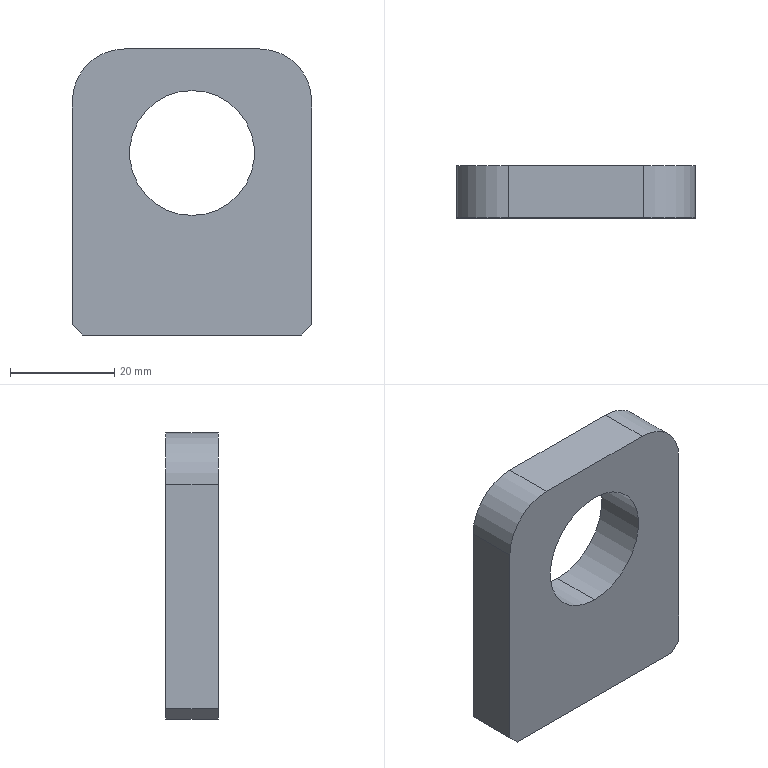Part | SolidWorks | features HoleWzd 2, Chamfer 1, Extrusion 1, Fillet 1 | 1 solid | 20 faces | box 46 x 10 x 55 mm | volume 20105 mm3 | cylinder 8 | plane 8 | cone 4 | commonest cylinder face diameters 3.3 x4 20 x2 24 x2
STEP:
#1=CARTESIAN_POINT('',(16.65,0.,-16.));
#2=VERTEX_POINT('',#1);
#3=CARTESIAN_POINT('',(13.35,0.,-16.));
#4=VERTEX_POINT('',#3);
#5=CARTESIAN_POINT('',(15.,0.,-16.));
#6=DIRECTION('',(0.,0.,-1.));
#7=DIRECTION('',(-1.,0.,0.));
#8=AXIS2_PLACEMENT_3D('',#5,#6,#7);
#9=CIRCLE('',#8,1.65);
#10=EDGE_CURVE('',#2,#4,#9,.T.);
#11=ORIENTED_EDGE('',*,*,#10,.F.);
#12=CARTESIAN_POINT('',(16.65,0.,-27.5));
#13=VERTEX_POINT('',#12);
#14=CARTESIAN_POINT('',(16.65,0.,-27.5));
#15=DIRECTION('',(0.,0.,-1.));
#16=VECTOR('',#15,1000.);
#17=LINE('',#14,#16);
#18=EDGE_CURVE('',#2,#13,#17,.T.);
#19=ORIENTED_EDGE('',*,*,#18,.T.);
#20=CARTESIAN_POINT('',(13.35,0.,-27.5));
#21=VERTEX_POINT('',#20);
#22=CARTESIAN_POINT('',(15.,0.,-27.5));
#23=DIRECTION('',(0.,0.,-1.));
#24=DIRECTION('',(-1.,0.,0.));
#25=AXIS2_PLACEMENT_3D('',#22,#23,#24);
#26=CIRCLE('',#25,1.65);
#27=EDGE_CURVE('',#13,#21,#26,.T.);
#28=ORIENTED_EDGE('',*,*,#27,.T.);
#29=CARTESIAN_POINT('',(13.35,0.,-27.5));
#30=DIRECTION('',(0.,0.,-1.));
#31=VECTOR('',#30,1000.);
#32=LINE('',#29,#31);
#33=EDGE_CURVE('',#4,#21,#32,.T.);
#34=ORIENTED_EDGE('',*,*,#33,.F.);
#35=EDGE_LOOP('',(#11,#19,#28,#34));
#36=FACE_OUTER_BOUND('',#35,.T.);
#37=CARTESIAN_POINT('',(15.,0.,-27.5));
#38=DIRECTION('',(0.,0.,-1.));
#39=DIRECTION('',(-1.,0.,0.));
#40=AXIS2_PLACEMENT_3D('',#37,#38,#39);
#41=CYLINDRICAL_SURFACE('',#40,1.65);
#42=ADVANCED_FACE('',(#36),#41,.F.);
#43=CARTESIAN_POINT('',(15.,0.,-15.009));
#44=VERTEX_POINT('',#43);
#45=CARTESIAN_POINT('',(13.35,0.,-16.));
#46=DIRECTION('',(-0.8572,0.,-0.515));
#47=VECTOR('',#46,1000.);
#48=LINE('',#45,#47);
#49=EDGE_CURVE('',#44,#4,#48,.T.);
#50=ORIENTED_EDGE('',*,*,#49,.F.);
#51=CARTESIAN_POINT('',(16.65,0.,-16.));
#52=DIRECTION('',(0.8572,0.,-0.515));
#53=VECTOR('',#52,1000.);
#54=LINE('',#51,#53);
#55=EDGE_CURVE('',#44,#2,#54,.T.);
#56=ORIENTED_EDGE('',*,*,#55,.T.);
#57=ORIENTED_EDGE('',*,*,#10,.T.);
#58=EDGE_LOOP('',(#50,#56,#57));
#59=FACE_OUTER_BOUND('',#58,.T.);
#60=CARTESIAN_POINT('',(15.,0.,-16.));
#61=DIRECTION('',(0.,0.,-1.));
#62=DIRECTION('',(-1.,0.,0.));
#63=AXIS2_PLACEMENT_3D('',#60,#61,#62);
#64=CONICAL_SURFACE('',#63,1.65,1.03);
#65=ADVANCED_FACE('',(#59),#64,.F.);
#66=CARTESIAN_POINT('',(-13.35,0.,-16.));
#67=VERTEX_POINT('',#66);
#68=CARTESIAN_POINT('',(-16.65,0.,-16.));
#69=VERTEX_POINT('',#68);
#70=CARTESIAN_POINT('',(-15.,0.,-16.));
#71=DIRECTION('',(0.,0.,-1.));
#72=DIRECTION('',(-1.,0.,0.));
#73=AXIS2_PLACEMENT_3D('',#70,#71,#72);
#74=CIRCLE('',#73,1.65);
#75=EDGE_CURVE('',#67,#69,#74,.T.);
#76=ORIENTED_EDGE('',*,*,#75,.F.);
#77=CARTESIAN_POINT('',(-13.35,0.,-27.5));
#78=VERTEX_POINT('',#77);
#79=CARTESIAN_POINT('',(-13.35,0.,-27.5));
#80=DIRECTION('',(0.,0.,-1.));
#81=VECTOR('',#80,1000.);
#82=LINE('',#79,#81);
#83=EDGE_CURVE('',#67,#78,#82,.T.);
#84=ORIENTED_EDGE('',*,*,#83,.T.);
#85=CARTESIAN_POINT('',(-16.65,0.,-27.5));
#86=VERTEX_POINT('',#85);
#87=CARTESIAN_POINT('',(-15.,0.,-27.5));
#88=DIRECTION('',(0.,0.,-1.));
#89=DIRECTION('',(-1.,0.,0.));
#90=AXIS2_PLACEMENT_3D('',#87,#88,#89);
#91=CIRCLE('',#90,1.65);
#92=EDGE_CURVE('',#78,#86,#91,.T.);
#93=ORIENTED_EDGE('',*,*,#92,.T.);
#94=CARTESIAN_POINT('',(-16.65,0.,-27.5));
#95=DIRECTION('',(0.,0.,-1.));
#96=VECTOR('',#95,1000.);
#97=LINE('',#94,#96);
#98=EDGE_CURVE('',#69,#86,#97,.T.);
#99=ORIENTED_EDGE('',*,*,#98,.F.);
#100=EDGE_LOOP('',(#76,#84,#93,#99));
#101=FACE_OUTER_BOUND('',#100,.T.);
#102=CARTESIAN_POINT('',(-15.,0.,-27.5));
#103=DIRECTION('',(0.,0.,-1.));
#104=DIRECTION('',(-1.,0.,0.));
#105=AXIS2_PLACEMENT_3D('',#102,#103,#104);
#106=CYLINDRICAL_SURFACE('',#105,1.65);
#107=ADVANCED_FACE('',(#101),#106,.F.);
#108=CARTESIAN_POINT('',(-15.,0.,-15.009));
#109=VERTEX_POINT('',#108);
#110=CARTESIAN_POINT('',(-16.65,0.,-16.));
#111=DIRECTION('',(-0.8572,0.,-0.515));
#112=VECTOR('',#111,1000.);
#113=LINE('',#110,#112);
#114=EDGE_CURVE('',#109,#69,#113,.T.);
#115=ORIENTED_EDGE('',*,*,#114,.F.);
#116=CARTESIAN_POINT('',(-13.35,0.,-16.));
#117=DIRECTION('',(0.8572,0.,-0.515));
#118=VECTOR('',#117,1000.);
#119=LINE('',#116,#118);
#120=EDGE_CURVE('',#109,#67,#119,.T.);
#121=ORIENTED_EDGE('',*,*,#120,.T.);
#122=ORIENTED_EDGE('',*,*,#75,.T.);
#123=EDGE_LOOP('',(#115,#121,#122));
#124=FACE_OUTER_BOUND('',#123,.T.);
#125=CARTESIAN_POINT('',(-15.,0.,-16.));
#126=DIRECTION('',(0.,0.,-1.));
#127=DIRECTION('',(-1.,0.,0.));
#128=AXIS2_PLACEMENT_3D('',#125,#126,#127);
#129=CONICAL_SURFACE('',#128,1.65,1.03);
#130=ADVANCED_FACE('',(#124),#129,.F.);
#131=CARTESIAN_POINT('',(0.,-5.,-4.5));
#132=VERTEX_POINT('',#131);
#133=CARTESIAN_POINT('',(0.,-5.,19.5));
#134=VERTEX_POINT('',#133);
#135=CARTESIAN_POINT('',(0.,-5.,7.5));
#136=DIRECTION('',(0.,1.,0.));
#137=DIRECTION('',(0.,0.,1.));
#138=AXIS2_PLACEMENT_3D('',#135,#136,#137);
#139=CIRCLE('',#138,12.);
#140=EDGE_CURVE('',#132,#134,#139,.T.);
#141=ORIENTED_EDGE('',*,*,#140,.F.);
#142=CARTESIAN_POINT('',(0.,5.,-4.5));
#143=VERTEX_POINT('',#142);
#144=CARTESIAN_POINT('',(0.,5.,-4.5));
#145=DIRECTION('',(0.,1.,0.));
#146=VECTOR('',#145,1000.);
#147=LINE('',#144,#146);
#148=EDGE_CURVE('',#132,#143,#147,.T.);
#149=ORIENTED_EDGE('',*,*,#148,.T.);
#150=CARTESIAN_POINT('',(0.,5.,19.5));
#151=VERTEX_POINT('',#150);
#152=CARTESIAN_POINT('',(0.,5.,7.5));
#153=DIRECTION('',(0.,1.,0.));
#154=DIRECTION('',(0.,0.,1.));
#155=AXIS2_PLACEMENT_3D('',#152,#153,#154);
#156=CIRCLE('',#155,12.);
#157=EDGE_CURVE('',#143,#151,#156,.T.);
#158=ORIENTED_EDGE('',*,*,#157,.T.);
#159=CARTESIAN_POINT('',(0.,5.,19.5));
#160=DIRECTION('',(0.,1.,0.));
#161=VECTOR('',#160,1000.);
#162=LINE('',#159,#161);
#163=EDGE_CURVE('',#134,#151,#162,.T.);
#164=ORIENTED_EDGE('',*,*,#163,.F.);
#165=EDGE_LOOP('',(#141,#149,#158,#164));
#166=FACE_OUTER_BOUND('',#165,.T.);
#167=CARTESIAN_POINT('',(0.,5.,7.5));
#168=DIRECTION('',(0.,1.,0.));
#169=DIRECTION('',(0.,0.,1.));
#170=AXIS2_PLACEMENT_3D('',#167,#168,#169);
#171=CYLINDRICAL_SURFACE('',#170,12.);
#172=ADVANCED_FACE('',(#166),#171,.F.);
#173=CARTESIAN_POINT('',(23.,-5.,17.5));
#174=VERTEX_POINT('',#173);
#175=CARTESIAN_POINT('',(23.,-5.,-25.5));
#176=VERTEX_POINT('',#175);
#177=CARTESIAN_POINT('',(23.,-5.,-27.5));
#178=DIRECTION('',(0.,0.,-1.));
#179=VECTOR('',#178,1000.);
#180=LINE('',#177,#179);
#181=EDGE_CURVE('',#174,#176,#180,.T.);
#182=ORIENTED_EDGE('',*,*,#181,.T.);
#183=CARTESIAN_POINT('',(23.,5.,-25.5));
#184=VERTEX_POINT('',#183);
#185=CARTESIAN_POINT('',(23.,5.,-25.5));
#186=DIRECTION('',(0.,1.,0.));
#187=VECTOR('',#186,1000.);
#188=LINE('',#185,#187);
#189=EDGE_CURVE('',#176,#184,#188,.T.);
#190=ORIENTED_EDGE('',*,*,#189,.T.);
#191=CARTESIAN_POINT('',(23.,5.,17.5));
#192=VERTEX_POINT('',#191);
#193=CARTESIAN_POINT('',(23.,5.,-27.5));
#194=DIRECTION('',(0.,0.,-1.));
#195=VECTOR('',#194,1000.);
#196=LINE('',#193,#195);
#197=EDGE_CURVE('',#192,#184,#196,.T.);
#198=ORIENTED_EDGE('',*,*,#197,.F.);
#199=CARTESIAN_POINT('',(23.,5.,17.5));
#200=DIRECTION('',(0.,-1.,0.));
#201=VECTOR('',#200,1000.);
#202=LINE('',#199,#201);
#203=EDGE_CURVE('',#192,#174,#202,.T.);
#204=ORIENTED_EDGE('',*,*,#203,.T.);
#205=EDGE_LOOP('',(#182,#190,#198,#204));
#206=FACE_OUTER_BOUND('',#205,.T.);
#207=CARTESIAN_POINT('',(23.,5.,-27.5));
#208=DIRECTION('',(-1.,0.,0.));
#209=DIRECTION('',(0.,0.,1.));
#210=AXIS2_PLACEMENT_3D('',#207,#208,#209);
#211=PLANE('',#210);
#212=ADVANCED_FACE('',(#206),#211,.F.);
#213=CARTESIAN_POINT('',(15.,0.,-27.5));
#214=DIRECTION('',(0.,0.,-1.));
#215=DIRECTION('',(-1.,0.,0.));
#216=AXIS2_PLACEMENT_3D('',#213,#214,#215);
#217=CIRCLE('',#216,1.65);
#218=EDGE_CURVE('',#21,#13,#217,.T.);
#219=ORIENTED_EDGE('',*,*,#218,.F.);
#220=ORIENTED_EDGE('',*,*,#27,.F.);
#221=EDGE_LOOP('',(#219,#220));
#222=FACE_BOUND('',#221,.T.);
#223=CARTESIAN_POINT('',(-15.,0.,-27.5));
#224=DIRECTION('',(0.,0.,-1.));
#225=DIRECTION('',(-1.,0.,0.));
#226=AXIS2_PLACEMENT_3D('',#223,#224,#225);
#227=CIRCLE('',#226,1.65);
#228=EDGE_CURVE('',#86,#78,#227,.T.);
#229=ORIENTED_EDGE('',*,*,#228,.F.);
#230=ORIENTED_EDGE('',*,*,#92,.F.);
#231=EDGE_LOOP('',(#229,#230));
#232=FACE_BOUND('',#231,.T.);
#233=CARTESIAN_POINT('',(21.,5.,-27.5));
#234=VERTEX_POINT('',#233);
#235=CARTESIAN_POINT('',(-21.,5.,-27.5));
#236=VERTEX_POINT('',#235);
#237=CARTESIAN_POINT('',(-23.,5.,-27.5));
#238=DIRECTION('',(-1.,0.,0.));
#239=VECTOR('',#238,1000.);
#240=LINE('',#237,#239);
#241=EDGE_CURVE('',#234,#236,#240,.T.);
#242=ORIENTED_EDGE('',*,*,#241,.F.);
#243=CARTESIAN_POINT('',(21.,-5.,-27.5));
#244=VERTEX_POINT('',#243);
#245=CARTESIAN_POINT('',(21.,5.,-27.5));
#246=DIRECTION('',(0.,-1.,0.));
#247=VECTOR('',#246,1000.);
#248=LINE('',#245,#247);
#249=EDGE_CURVE('',#234,#244,#248,.T.);
#250=ORIENTED_EDGE('',*,*,#249,.T.);
#251=CARTESIAN_POINT('',(-21.,-5.,-27.5));
#252=VERTEX_POINT('',#251);
#253=CARTESIAN_POINT('',(-23.,-5.,-27.5));
#254=DIRECTION('',(-1.,0.,0.));
#255=VECTOR('',#254,1000.);
#256=LINE('',#253,#255);
#257=EDGE_CURVE('',#244,#252,#256,.T.);
#258=ORIENTED_EDGE('',*,*,#257,.T.);
#259=CARTESIAN_POINT('',(-21.,5.,-27.5));
#260=DIRECTION('',(0.,1.,0.));
#261=VECTOR('',#260,1000.);
#262=LINE('',#259,#261);
#263=EDGE_CURVE('',#252,#236,#262,.T.);
#264=ORIENTED_EDGE('',*,*,#263,.T.);
#265=EDGE_LOOP('',(#242,#250,#258,#264));
#266=FACE_OUTER_BOUND('',#265,.T.);
#267=CARTESIAN_POINT('',(-23.,5.,-27.5));
#268=DIRECTION('',(0.,0.,1.));
#269=DIRECTION('',(1.,0.,0.));
#270=AXIS2_PLACEMENT_3D('',#267,#268,#269);
#271=PLANE('',#270);
#272=ADVANCED_FACE('',(#222,#232,#266),#271,.F.);
#273=CARTESIAN_POINT('',(-23.,5.,-25.5));
#274=VERTEX_POINT('',#273);
#275=CARTESIAN_POINT('',(-23.,5.,17.5));
#276=VERTEX_POINT('',#275);
#277=CARTESIAN_POINT('',(-23.,5.,-27.5));
#278=DIRECTION('',(0.,0.,1.));
#279=VECTOR('',#278,1000.);
#280=LINE('',#277,#279);
#281=EDGE_CURVE('',#274,#276,#280,.T.);
#282=ORIENTED_EDGE('',*,*,#281,.F.);
#283=CARTESIAN_POINT('',(-23.,-5.,-25.5));
#284=VERTEX_POINT('',#283);
#285=CARTESIAN_POINT('',(-23.,5.,-25.5));
#286=DIRECTION('',(0.,-1.,0.));
#287=VECTOR('',#286,1000.);
#288=LINE('',#285,#287);
#289=EDGE_CURVE('',#274,#284,#288,.T.);
#290=ORIENTED_EDGE('',*,*,#289,.T.);
#291=CARTESIAN_POINT('',(-23.,-5.,17.5));
#292=VERTEX_POINT('',#291);
#293=CARTESIAN_POINT('',(-23.,-5.,-27.5));
#294=DIRECTION('',(0.,0.,1.));
#295=VECTOR('',#294,1000.);
#296=LINE('',#293,#295);
#297=EDGE_CURVE('',#284,#292,#296,.T.);
#298=ORIENTED_EDGE('',*,*,#297,.T.);
#299=CARTESIAN_POINT('',(-23.,5.,17.5));
#300=DIRECTION('',(0.,1.,0.));
#301=VECTOR('',#300,1000.);
#302=LINE('',#299,#301);
#303=EDGE_CURVE('',#292,#276,#302,.T.);
#304=ORIENTED_EDGE('',*,*,#303,.T.);
#305=EDGE_LOOP('',(#282,#290,#298,#304));
#306=FACE_OUTER_BOUND('',#305,.T.);
#307=CARTESIAN_POINT('',(-23.,5.,-27.5));
#308=DIRECTION('',(1.,0.,0.));
#309=DIRECTION('',(0.,0.,-1.));
#310=AXIS2_PLACEMENT_3D('',#307,#308,#309);
#311=PLANE('',#310);
#312=ADVANCED_FACE('',(#306),#311,.F.);
#313=CARTESIAN_POINT('',(-13.,-5.,27.5));
#314=VERTEX_POINT('',#313);
#315=CARTESIAN_POINT('',(13.,-5.,27.5));
#316=VERTEX_POINT('',#315);
#317=CARTESIAN_POINT('',(-23.,-5.,27.5));
#318=DIRECTION('',(1.,0.,0.));
#319=VECTOR('',#318,1000.);
#320=LINE('',#317,#319);
#321=EDGE_CURVE('',#314,#316,#320,.T.);
#322=ORIENTED_EDGE('',*,*,#321,.T.);
#323=CARTESIAN_POINT('',(13.,5.,27.5));
#324=VERTEX_POINT('',#323);
#325=CARTESIAN_POINT('',(13.,5.,27.5));
#326=DIRECTION('',(0.,1.,0.));
#327=VECTOR('',#326,1000.);
#328=LINE('',#325,#327);
#329=EDGE_CURVE('',#316,#324,#328,.T.);
#330=ORIENTED_EDGE('',*,*,#329,.T.);
#331=CARTESIAN_POINT('',(-13.,5.,27.5));
#332=VERTEX_POINT('',#331);
#333=CARTESIAN_POINT('',(-23.,5.,27.5));
#334=DIRECTION('',(1.,0.,0.));
#335=VECTOR('',#334,1000.);
#336=LINE('',#333,#335);
#337=EDGE_CURVE('',#332,#324,#336,.T.);
#338=ORIENTED_EDGE('',*,*,#337,.F.);
#339=CARTESIAN_POINT('',(-13.,5.,27.5));
#340=DIRECTION('',(0.,-1.,0.));
#341=VECTOR('',#340,1000.);
#342=LINE('',#339,#341);
#343=EDGE_CURVE('',#332,#314,#342,.T.);
#344=ORIENTED_EDGE('',*,*,#343,.T.);
#345=EDGE_LOOP('',(#322,#330,#338,#344));
#346=FACE_OUTER_BOUND('',#345,.T.);
#347=CARTESIAN_POINT('',(-23.,5.,27.5));
#348=DIRECTION('',(0.,0.,-1.));
#349=DIRECTION('',(-1.,0.,0.));
#350=AXIS2_PLACEMENT_3D('',#347,#348,#349);
#351=PLANE('',#350);
#352=ADVANCED_FACE('',(#346),#351,.F.);
#353=CARTESIAN_POINT('',(0.,5.,7.5));
#354=DIRECTION('',(0.,1.,0.));
#355=DIRECTION('',(0.,0.,1.));
#356=AXIS2_PLACEMENT_3D('',#353,#354,#355);
#357=CIRCLE('',#356,12.);
#358=EDGE_CURVE('',#151,#143,#357,.T.);
#359=ORIENTED_EDGE('',*,*,#358,.F.);
#360=ORIENTED_EDGE('',*,*,#157,.F.);
#361=EDGE_LOOP('',(#359,#360));
#362=FACE_BOUND('',#361,.T.);
#363=ORIENTED_EDGE('',*,*,#197,.T.);
#364=CARTESIAN_POINT('',(24.25,5.,-24.25));
#365=DIRECTION('',(-0.7071,0.,-0.7071));
#366=VECTOR('',#365,1000.);
#367=LINE('',#364,#366);
#368=EDGE_CURVE('',#184,#234,#367,.T.);
#369=ORIENTED_EDGE('',*,*,#368,.T.);
#370=ORIENTED_EDGE('',*,*,#241,.T.);
#371=CARTESIAN_POINT('',(-24.25,5.,-24.25));
#372=DIRECTION('',(-0.7071,0.,0.7071));
#373=VECTOR('',#372,1000.);
#374=LINE('',#371,#373);
#375=EDGE_CURVE('',#236,#274,#374,.T.);
#376=ORIENTED_EDGE('',*,*,#375,.T.);
#377=ORIENTED_EDGE('',*,*,#281,.T.);
#378=CARTESIAN_POINT('',(-13.,5.,17.5));
#379=DIRECTION('',(0.,1.,0.));
#380=DIRECTION('',(0.,0.,1.));
#381=AXIS2_PLACEMENT_3D('',#378,#379,#380);
#382=CIRCLE('',#381,10.);
#383=EDGE_CURVE('',#276,#332,#382,.T.);
#384=ORIENTED_EDGE('',*,*,#383,.T.);
#385=ORIENTED_EDGE('',*,*,#337,.T.);
#386=CARTESIAN_POINT('',(13.,5.,17.5));
#387=DIRECTION('',(0.,1.,0.));
#388=DIRECTION('',(0.,0.,1.));
#389=AXIS2_PLACEMENT_3D('',#386,#387,#388);
#390=CIRCLE('',#389,10.);
#391=EDGE_CURVE('',#324,#192,#390,.T.);
#392=ORIENTED_EDGE('',*,*,#391,.T.);
#393=EDGE_LOOP('',(#363,#369,#370,#376,#377,#384,#385,#392));
#394=FACE_OUTER_BOUND('',#393,.T.);
#395=CARTESIAN_POINT('',(0.,5.,0.));
#396=DIRECTION('',(0.,1.,0.));
#397=DIRECTION('',(0.,0.,1.));
#398=AXIS2_PLACEMENT_3D('',#395,#396,#397);
#399=PLANE('',#398);
#400=ADVANCED_FACE('',(#362,#394),#399,.T.);
#401=CARTESIAN_POINT('',(0.,-5.,7.5));
#402=DIRECTION('',(0.,1.,0.));
#403=DIRECTION('',(0.,0.,1.));
#404=AXIS2_PLACEMENT_3D('',#401,#402,#403);
#405=CIRCLE('',#404,12.);
#406=EDGE_CURVE('',#134,#132,#405,.T.);
#407=ORIENTED_EDGE('',*,*,#406,.T.);
#408=ORIENTED_EDGE('',*,*,#140,.T.);
#409=EDGE_LOOP('',(#407,#408));
#410=FACE_BOUND('',#409,.T.);
#411=ORIENTED_EDGE('',*,*,#257,.F.);
#412=CARTESIAN_POINT('',(21.,-5.,-27.5));
#413=DIRECTION('',(0.7071,0.,0.7071));
#414=VECTOR('',#413,1000.);
#415=LINE('',#412,#414);
#416=EDGE_CURVE('',#244,#176,#415,.T.);
#417=ORIENTED_EDGE('',*,*,#416,.T.);
#418=ORIENTED_EDGE('',*,*,#181,.F.);
#419=CARTESIAN_POINT('',(13.,-5.,17.5));
#420=DIRECTION('',(0.,-1.,0.));
#421=DIRECTION('',(0.,0.,1.));
#422=AXIS2_PLACEMENT_3D('',#419,#420,#421);
#423=CIRCLE('',#422,10.);
#424=EDGE_CURVE('',#174,#316,#423,.T.);
#425=ORIENTED_EDGE('',*,*,#424,.T.);
#426=ORIENTED_EDGE('',*,*,#321,.F.);
#427=CARTESIAN_POINT('',(-13.,-5.,17.5));
#428=DIRECTION('',(0.,-1.,0.));
#429=DIRECTION('',(0.,0.,1.));
#430=AXIS2_PLACEMENT_3D('',#427,#428,#429);
#431=CIRCLE('',#430,10.);
#432=EDGE_CURVE('',#314,#292,#431,.T.);
#433=ORIENTED_EDGE('',*,*,#432,.T.);
#434=ORIENTED_EDGE('',*,*,#297,.F.);
#435=CARTESIAN_POINT('',(-23.,-5.,-25.5));
#436=DIRECTION('',(0.7071,0.,-0.7071));
#437=VECTOR('',#436,1000.);
#438=LINE('',#435,#437);
#439=EDGE_CURVE('',#284,#252,#438,.T.);
#440=ORIENTED_EDGE('',*,*,#439,.T.);
#441=EDGE_LOOP('',(#411,#417,#418,#425,#426,#433,#434,#440));
#442=FACE_OUTER_BOUND('',#441,.T.);
#443=CARTESIAN_POINT('',(0.,-5.,0.));
#444=DIRECTION('',(0.,1.,0.));
#445=DIRECTION('',(0.,0.,1.));
#446=AXIS2_PLACEMENT_3D('',#443,#444,#445);
#447=PLANE('',#446);
#448=ADVANCED_FACE('',(#410,#442),#447,.F.);
#449=ORIENTED_EDGE('',*,*,#148,.F.);
#450=ORIENTED_EDGE('',*,*,#406,.F.);
#451=ORIENTED_EDGE('',*,*,#163,.T.);
#452=ORIENTED_EDGE('',*,*,#358,.T.);
#453=EDGE_LOOP('',(#449,#450,#451,#452));
#454=FACE_OUTER_BOUND('',#453,.T.);
#455=CARTESIAN_POINT('',(0.,5.,7.5));
#456=DIRECTION('',(0.,1.,0.));
#457=DIRECTION('',(0.,0.,1.));
#458=AXIS2_PLACEMENT_3D('',#455,#456,#457);
#459=CYLINDRICAL_SURFACE('',#458,12.);
#460=ADVANCED_FACE('',(#454),#459,.F.);
#461=ORIENTED_EDGE('',*,*,#391,.F.);
#462=ORIENTED_EDGE('',*,*,#329,.F.);
#463=ORIENTED_EDGE('',*,*,#424,.F.);
#464=ORIENTED_EDGE('',*,*,#203,.F.);
#465=EDGE_LOOP('',(#461,#462,#463,#464));
#466=FACE_OUTER_BOUND('',#465,.T.);
#467=CARTESIAN_POINT('',(13.,5.,17.5));
#468=DIRECTION('',(0.,-1.,0.));
#469=DIRECTION('',(0.,0.,-1.));
#470=AXIS2_PLACEMENT_3D('',#467,#468,#469);
#471=CYLINDRICAL_SURFACE('',#470,10.);
#472=ADVANCED_FACE('',(#466),#471,.T.);
#473=ORIENTED_EDGE('',*,*,#383,.F.);
#474=ORIENTED_EDGE('',*,*,#303,.F.);
#475=ORIENTED_EDGE('',*,*,#432,.F.);
#476=ORIENTED_EDGE('',*,*,#343,.F.);
#477=EDGE_LOOP('',(#473,#474,#475,#476));
#478=FACE_OUTER_BOUND('',#477,.T.);
#479=CARTESIAN_POINT('',(-13.,5.,17.5));
#480=DIRECTION('',(0.,-1.,0.));
#481=DIRECTION('',(0.,0.,-1.));
#482=AXIS2_PLACEMENT_3D('',#479,#480,#481);
#483=CYLINDRICAL_SURFACE('',#482,10.);
#484=ADVANCED_FACE('',(#478),#483,.T.);
#485=ORIENTED_EDGE('',*,*,#120,.F.);
#486=ORIENTED_EDGE('',*,*,#114,.T.);
#487=CARTESIAN_POINT('',(-15.,0.,-16.));
#488=DIRECTION('',(0.,0.,-1.));
#489=DIRECTION('',(-1.,0.,0.));
#490=AXIS2_PLACEMENT_3D('',#487,#488,#489);
#491=CIRCLE('',#490,1.65);
#492=EDGE_CURVE('',#69,#67,#491,.T.);
#493=ORIENTED_EDGE('',*,*,#492,.T.);
#494=EDGE_LOOP('',(#485,#486,#493));
#495=FACE_OUTER_BOUND('',#494,.T.);
#496=CARTESIAN_POINT('',(-15.,0.,-16.));
#497=DIRECTION('',(0.,0.,-1.));
#498=DIRECTION('',(-1.,0.,0.));
#499=AXIS2_PLACEMENT_3D('',#496,#497,#498);
#500=CONICAL_SURFACE('',#499,1.65,1.03);
#501=ADVANCED_FACE('',(#495),#500,.F.);
#502=ORIENTED_EDGE('',*,*,#83,.F.);
#503=ORIENTED_EDGE('',*,*,#492,.F.);
#504=ORIENTED_EDGE('',*,*,#98,.T.);
#505=ORIENTED_EDGE('',*,*,#228,.T.);
#506=EDGE_LOOP('',(#502,#503,#504,#505));
#507=FACE_OUTER_BOUND('',#506,.T.);
#508=CARTESIAN_POINT('',(-15.,0.,-27.5));
#509=DIRECTION('',(0.,0.,-1.));
#510=DIRECTION('',(-1.,0.,0.));
#511=AXIS2_PLACEMENT_3D('',#508,#509,#510);
#512=CYLINDRICAL_SURFACE('',#511,1.65);
#513=ADVANCED_FACE('',(#507),#512,.F.);
#514=ORIENTED_EDGE('',*,*,#55,.F.);
#515=ORIENTED_EDGE('',*,*,#49,.T.);
#516=CARTESIAN_POINT('',(15.,0.,-16.));
#517=DIRECTION('',(0.,0.,-1.));
#518=DIRECTION('',(-1.,0.,0.));
#519=AXIS2_PLACEMENT_3D('',#516,#517,#518);
#520=CIRCLE('',#519,1.65);
#521=EDGE_CURVE('',#4,#2,#520,.T.);
#522=ORIENTED_EDGE('',*,*,#521,.T.);
#523=EDGE_LOOP('',(#514,#515,#522));
#524=FACE_OUTER_BOUND('',#523,.T.);
#525=CARTESIAN_POINT('',(15.,0.,-16.));
#526=DIRECTION('',(0.,0.,-1.));
#527=DIRECTION('',(-1.,0.,0.));
#528=AXIS2_PLACEMENT_3D('',#525,#526,#527);
#529=CONICAL_SURFACE('',#528,1.65,1.03);
#530=ADVANCED_FACE('',(#524),#529,.F.);
#531=ORIENTED_EDGE('',*,*,#18,.F.);
#532=ORIENTED_EDGE('',*,*,#521,.F.);
#533=ORIENTED_EDGE('',*,*,#33,.T.);
#534=ORIENTED_EDGE('',*,*,#218,.T.);
#535=EDGE_LOOP('',(#531,#532,#533,#534));
#536=FACE_OUTER_BOUND('',#535,.T.);
#537=CARTESIAN_POINT('',(15.,0.,-27.5));
#538=DIRECTION('',(0.,0.,-1.));
#539=DIRECTION('',(-1.,0.,0.));
#540=AXIS2_PLACEMENT_3D('',#537,#538,#539);
#541=CYLINDRICAL_SURFACE('',#540,1.65);
#542=ADVANCED_FACE('',(#536),#541,.F.);
#543=ORIENTED_EDGE('',*,*,#368,.F.);
#544=ORIENTED_EDGE('',*,*,#189,.F.);
#545=ORIENTED_EDGE('',*,*,#416,.F.);
#546=ORIENTED_EDGE('',*,*,#249,.F.);
#547=EDGE_LOOP('',(#543,#544,#545,#546));
#548=FACE_OUTER_BOUND('',#547,.T.);
#549=CARTESIAN_POINT('',(21.,5.,-27.5));
#550=DIRECTION('',(-0.7071,0.,0.7071));
#551=DIRECTION('',(0.,-1.,0.));
#552=AXIS2_PLACEMENT_3D('',#549,#550,#551);
#553=PLANE('',#552);
#554=ADVANCED_FACE('',(#548),#553,.F.);
#555=ORIENTED_EDGE('',*,*,#375,.F.);
#556=ORIENTED_EDGE('',*,*,#263,.F.);
#557=ORIENTED_EDGE('',*,*,#439,.F.);
#558=ORIENTED_EDGE('',*,*,#289,.F.);
#559=EDGE_LOOP('',(#555,#556,#557,#558));
#560=FACE_OUTER_BOUND('',#559,.T.);
#561=CARTESIAN_POINT('',(-23.,5.,-25.5));
#562=DIRECTION('',(0.7071,0.,0.7071));
#563=DIRECTION('',(0.,-1.,0.));
#564=AXIS2_PLACEMENT_3D('',#561,#562,#563);
#565=PLANE('',#564);
#566=ADVANCED_FACE('',(#560),#565,.F.);
#567=CLOSED_SHELL('',(#42,#65,#107,#130,#172,#212,#272,#312,#352,#400,#448,#460,#472,#484,#501,#513,#530,#542,#554,#566));
#568=MANIFOLD_SOLID_BREP('',#567);
#569=CARTESIAN_POINT('',(0.,0.,0.));
#570=DIRECTION('',(0.,0.,1.));
#571=DIRECTION('',(1.,0.,0.));
#572=AXIS2_PLACEMENT_3D('',#569,#570,#571);
#573=(LENGTH_UNIT()NAMED_UNIT(*)SI_UNIT(.MILLI.,.METRE.));
#574=UNCERTAINTY_MEASURE_WITH_UNIT(LENGTH_MEASURE(0.00001),#573,'','');
#575=(NAMED_UNIT(*)PLANE_ANGLE_UNIT()SI_UNIT($,.RADIAN.));
#576=(NAMED_UNIT(*)SI_UNIT($,.STERADIAN.)SOLID_ANGLE_UNIT());
#577=(GEOMETRIC_REPRESENTATION_CONTEXT(3)GLOBAL_UNCERTAINTY_ASSIGNED_CONTEXT((#574))GLOBAL_UNIT_ASSIGNED_CONTEXT((#573,#575,#576))REPRESENTATION_CONTEXT('',''));
#578=ADVANCED_BREP_SHAPE_REPRESENTATION('',(#568,#572),#577);